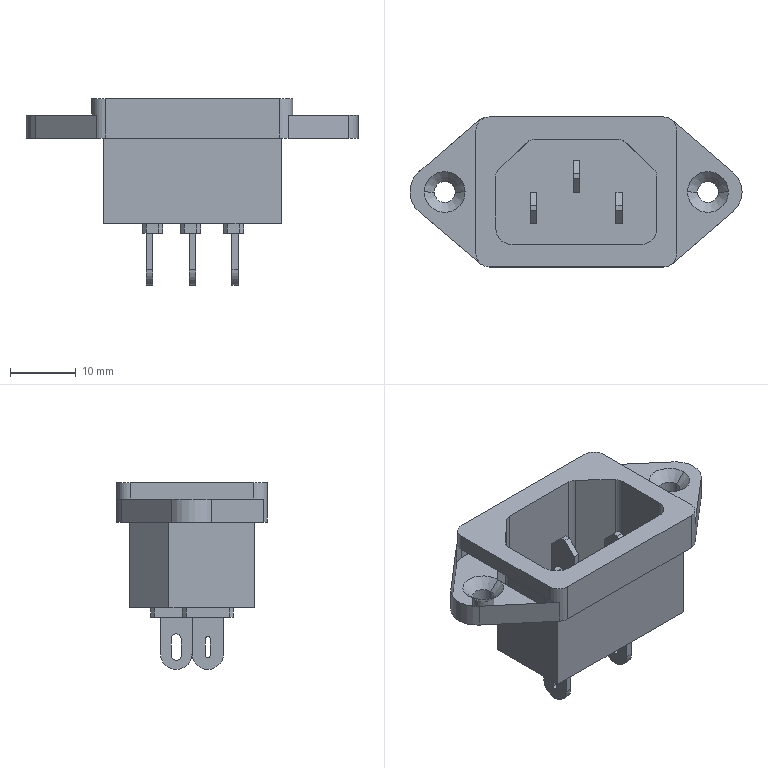Part | STEP file | AC220V three-pin socket-KET-301 | 4 solids | 324 faces | box 50.485 x 22.8 x 28.4 mm | volume 5143 mm3 | plane 234 | spline 54 | cylinder 32 | cone 4 | commonest cylinder face diameters 0.7 x6 4.8 x5 3 x4 3.2 x4 4 x4 1.5 x3